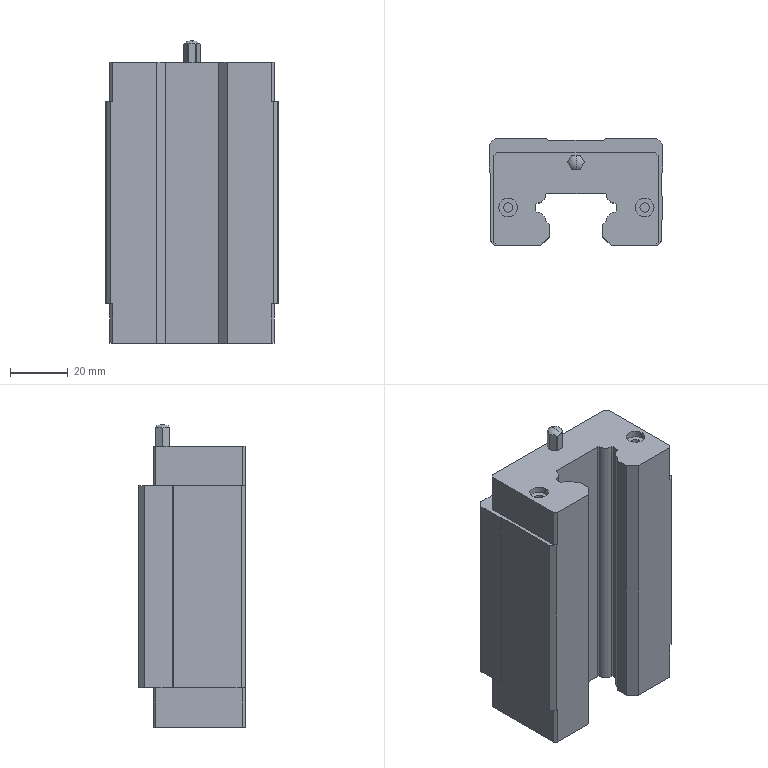Part | STEP file | _IBC23-45-100_002 | 1 solid | 125 faces | box 60 x 37 x 104.901 mm | volume 162215 mm3 | plane 71 | cylinder 36 | cone 16 | torus 2 | commonest cylinder face diameters 3.25 x8 6.5 x8 6.647 x8 0.4 x7 6.2 x4 10.1 x1